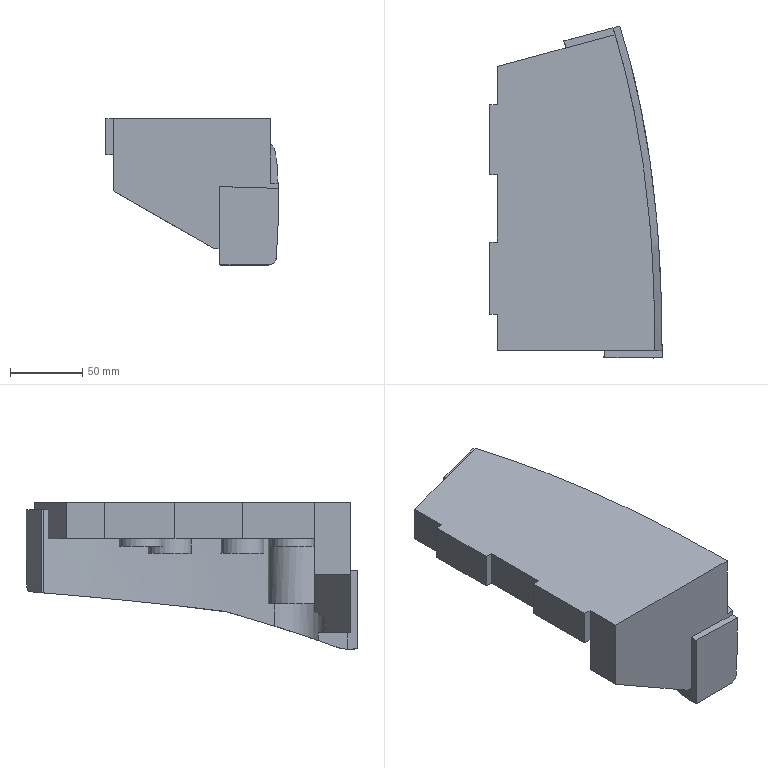Part | NX | features solid 2 | 1 solid | 58 faces | box 119.022 x 229.324 x 101.436 mm | volume 1150137 mm3 | spline 32 | plane 20 | cylinder 6 | commonest cylinder face diameters 30 x4 40 x2